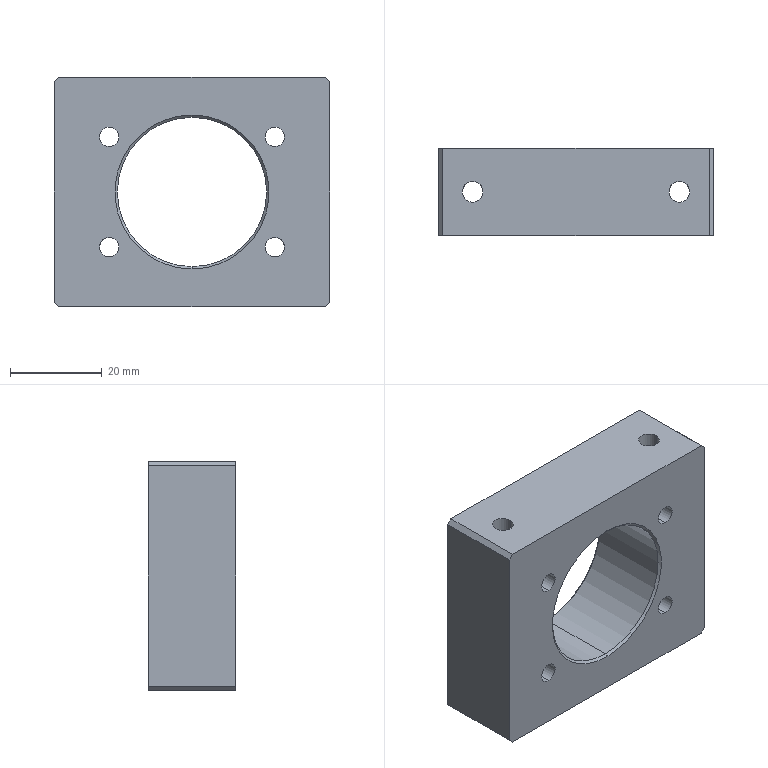Part | STEP file | 1 solid | 34 faces | box 60 x 19 x 50 mm | volume 36440 mm3 | cylinder 18 | plane 12 | cone 4 | commonest cylinder face diameters 4.2 x8 4.5 x4 8 x4 32.5 x2